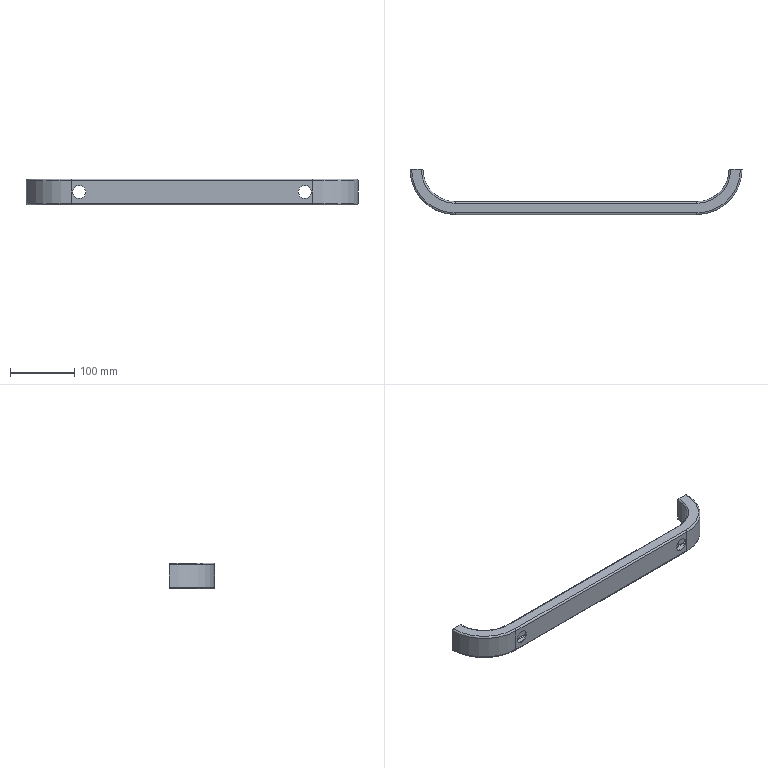Part | STEP file | 5091301 | 1 solid | 46 faces | box 515 x 70 x 40 mm | volume 91933 mm3 | cylinder 20 | torus 16 | plane 10 | commonest cylinder face diameters 2 x4 5 x4 20 x4 100 x2 103 x2 137 x2